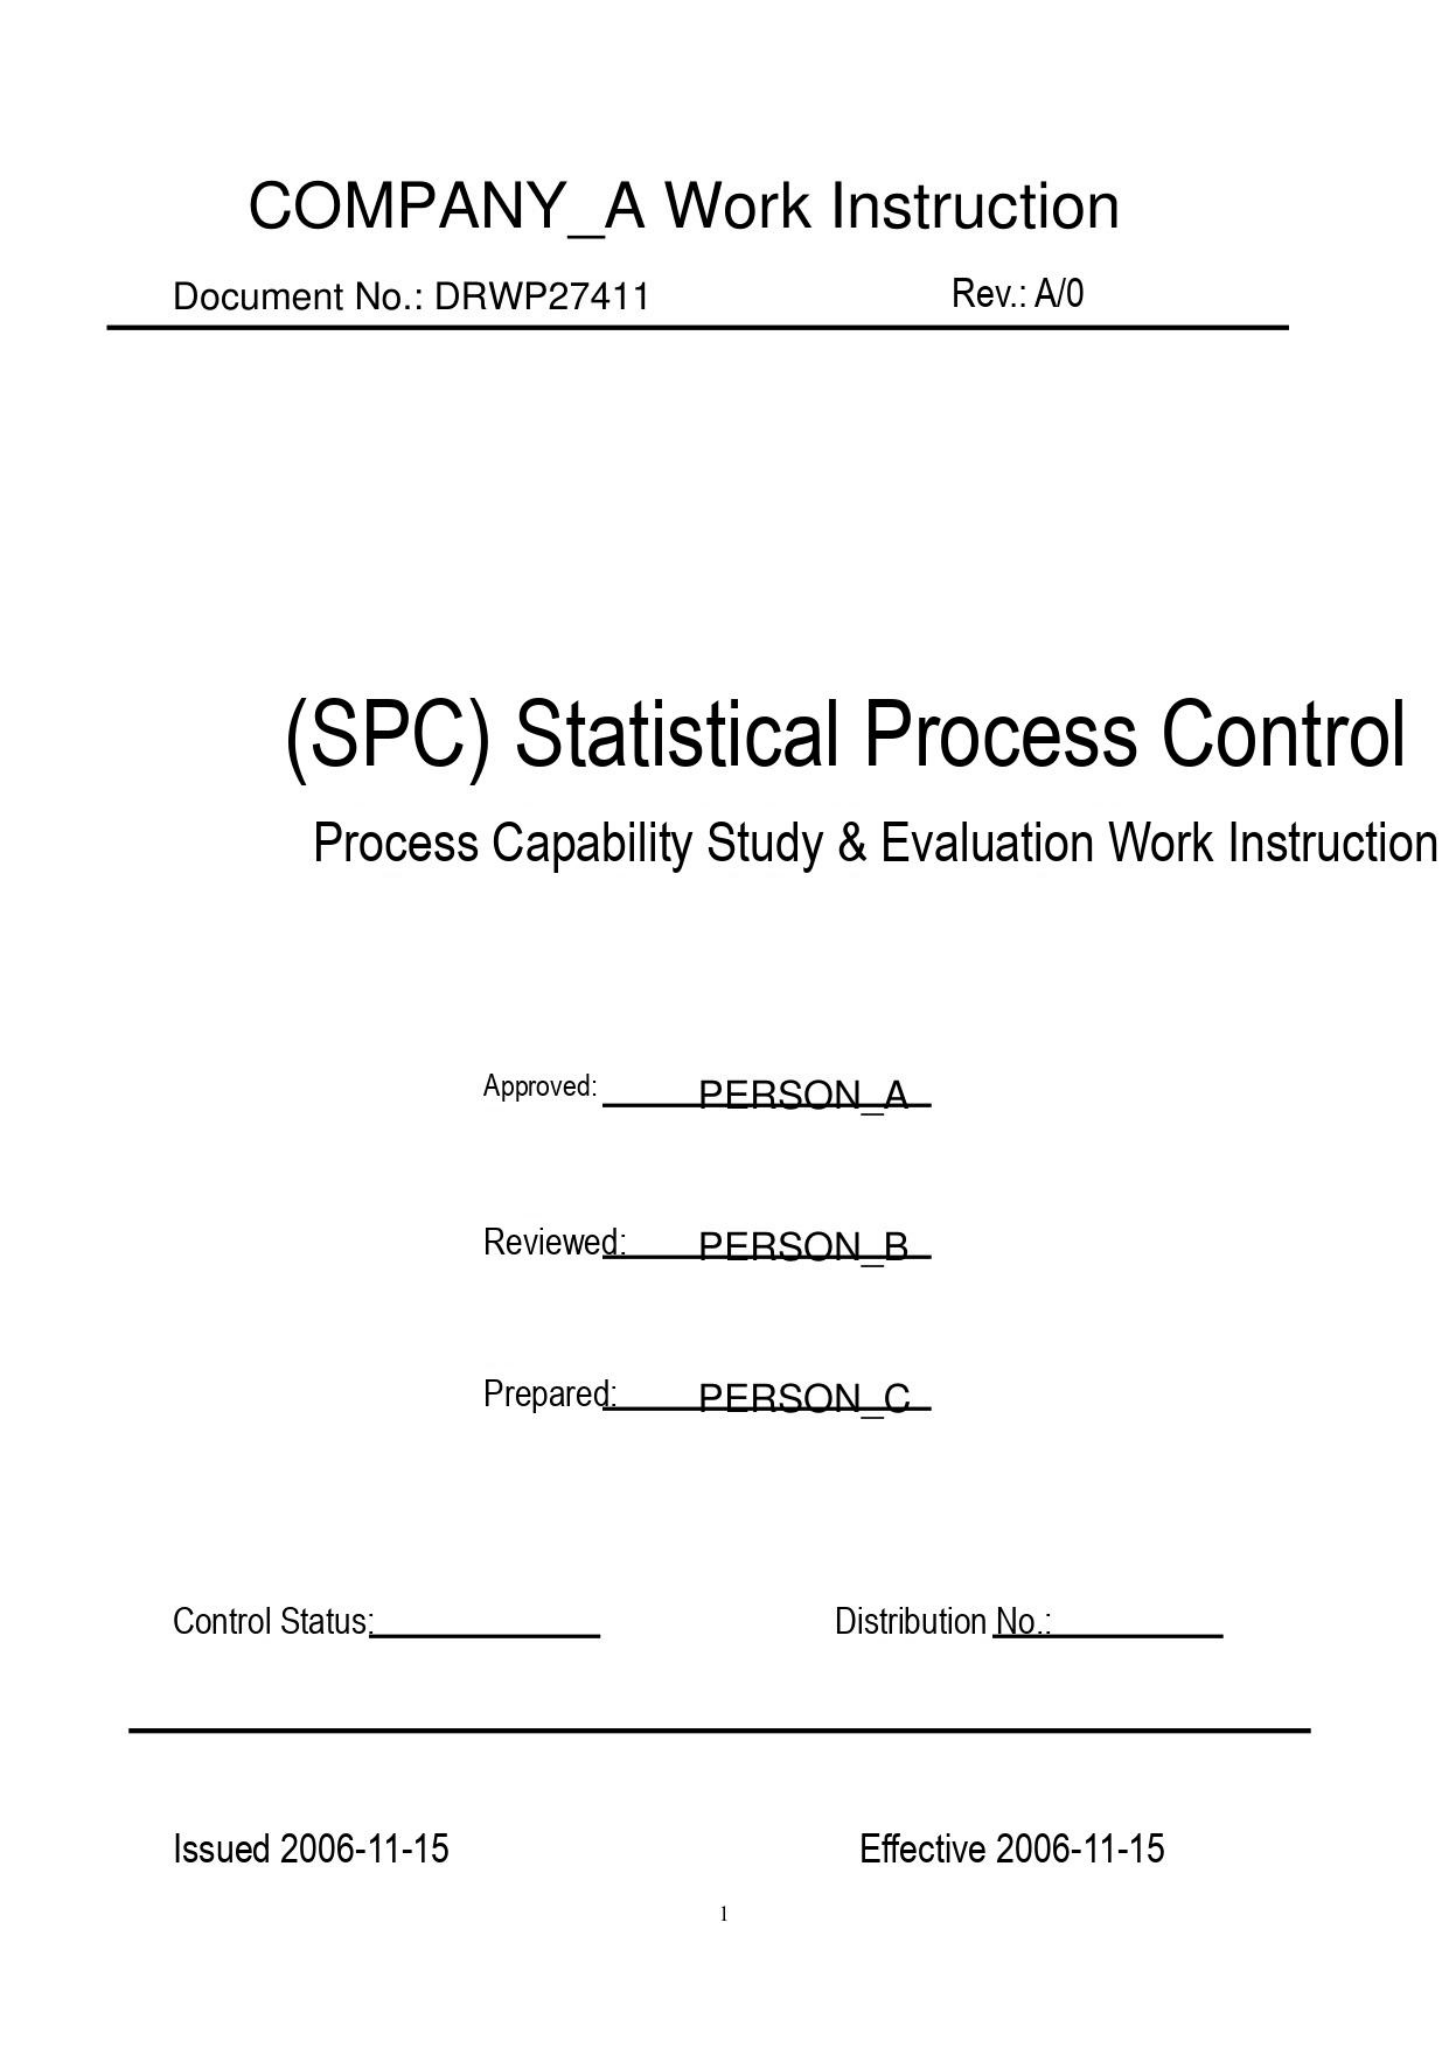COMPANY_A Work Instruction

Document No.: DRWP27411 Rev.: A/0

(SPC) Statistical Process Control

Process Capability Study & Evaluation Work Instruction

Approved: PERSON_A

Reviewed: PERSON_B

Prepared: PERSON_C

Control Status:

Distribution No.:

Issued 2006-11-15

Effective 2006-11-15

1
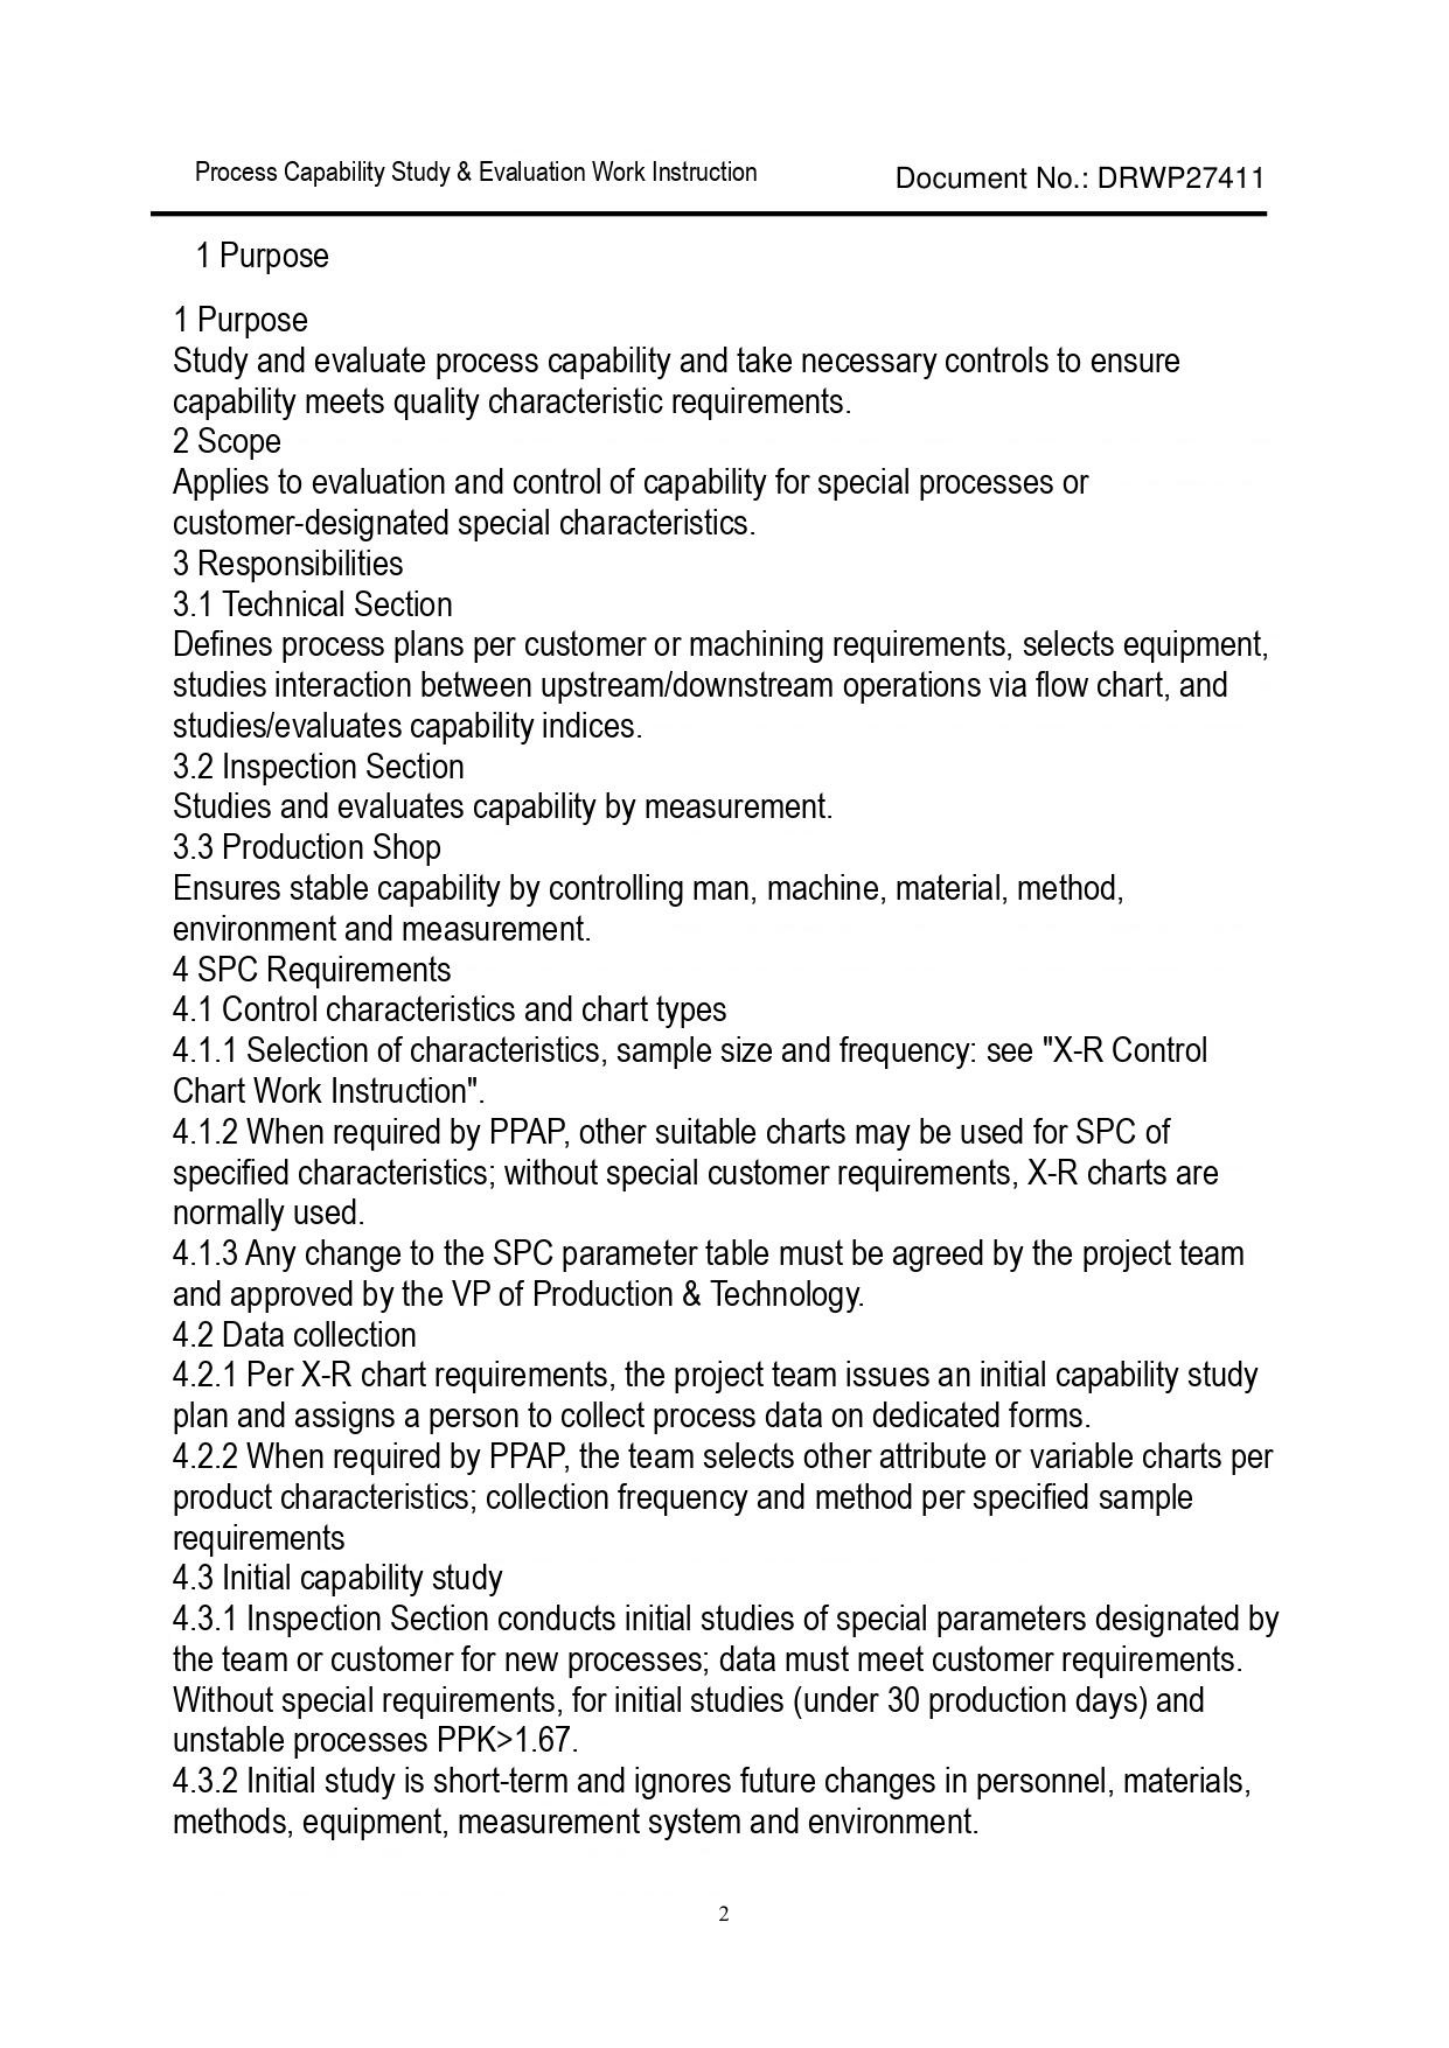Process Capability Study & Evaluation Work Instruction    Document No.: DRWP27411

1 Purpose

1 Purpose
Study and evaluate process capability and take necessary controls to ensure capability meets quality characteristic requirements.
2 Scope
Applies to evaluation and control of capability for special processes or customer-designated special characteristics.
3 Responsibilities
3.1 Technical Section
Defines process plans per customer or machining requirements, selects equipment, studies interaction between upstream/downstream operations via flow chart, and studies/evaluates capability indices.
3.2 Inspection Section
Studies and evaluates capability by measurement.
3.3 Production Shop
Ensures stable capability by controlling man, machine, material, method, environment and measurement.
4 SPC Requirements
4.1 Control characteristics and chart types
4.1.1 Selection of characteristics, sample size and frequency: see "X-R Control Chart Work Instruction".
4.1.2 When required by PPAP, other suitable charts may be used for SPC of specified characteristics; without special customer requirements, X-R charts are normally used.
4.1.3 Any change to the SPC parameter table must be agreed by the project team and approved by the VP of Production & Technology.
4.2 Data collection
4.2.1 Per X-R chart requirements, the project team issues an initial capability study plan and assigns a person to collect process data on dedicated forms.
4.2.2 When required by PPAP, the team selects other attribute or variable charts per product characteristics; collection frequency and method per specified sample requirements
4.3 Initial capability study
4.3.1 Inspection Section conducts initial studies of special parameters designated by the team or customer for new processes; data must meet customer requirements. Without special requirements, for initial studies (under 30 production days) and unstable processes PPK>1.67.
4.3.2 Initial study is short-term and ignores future changes in personnel, materials, methods, equipment, measurement system and environment.

2
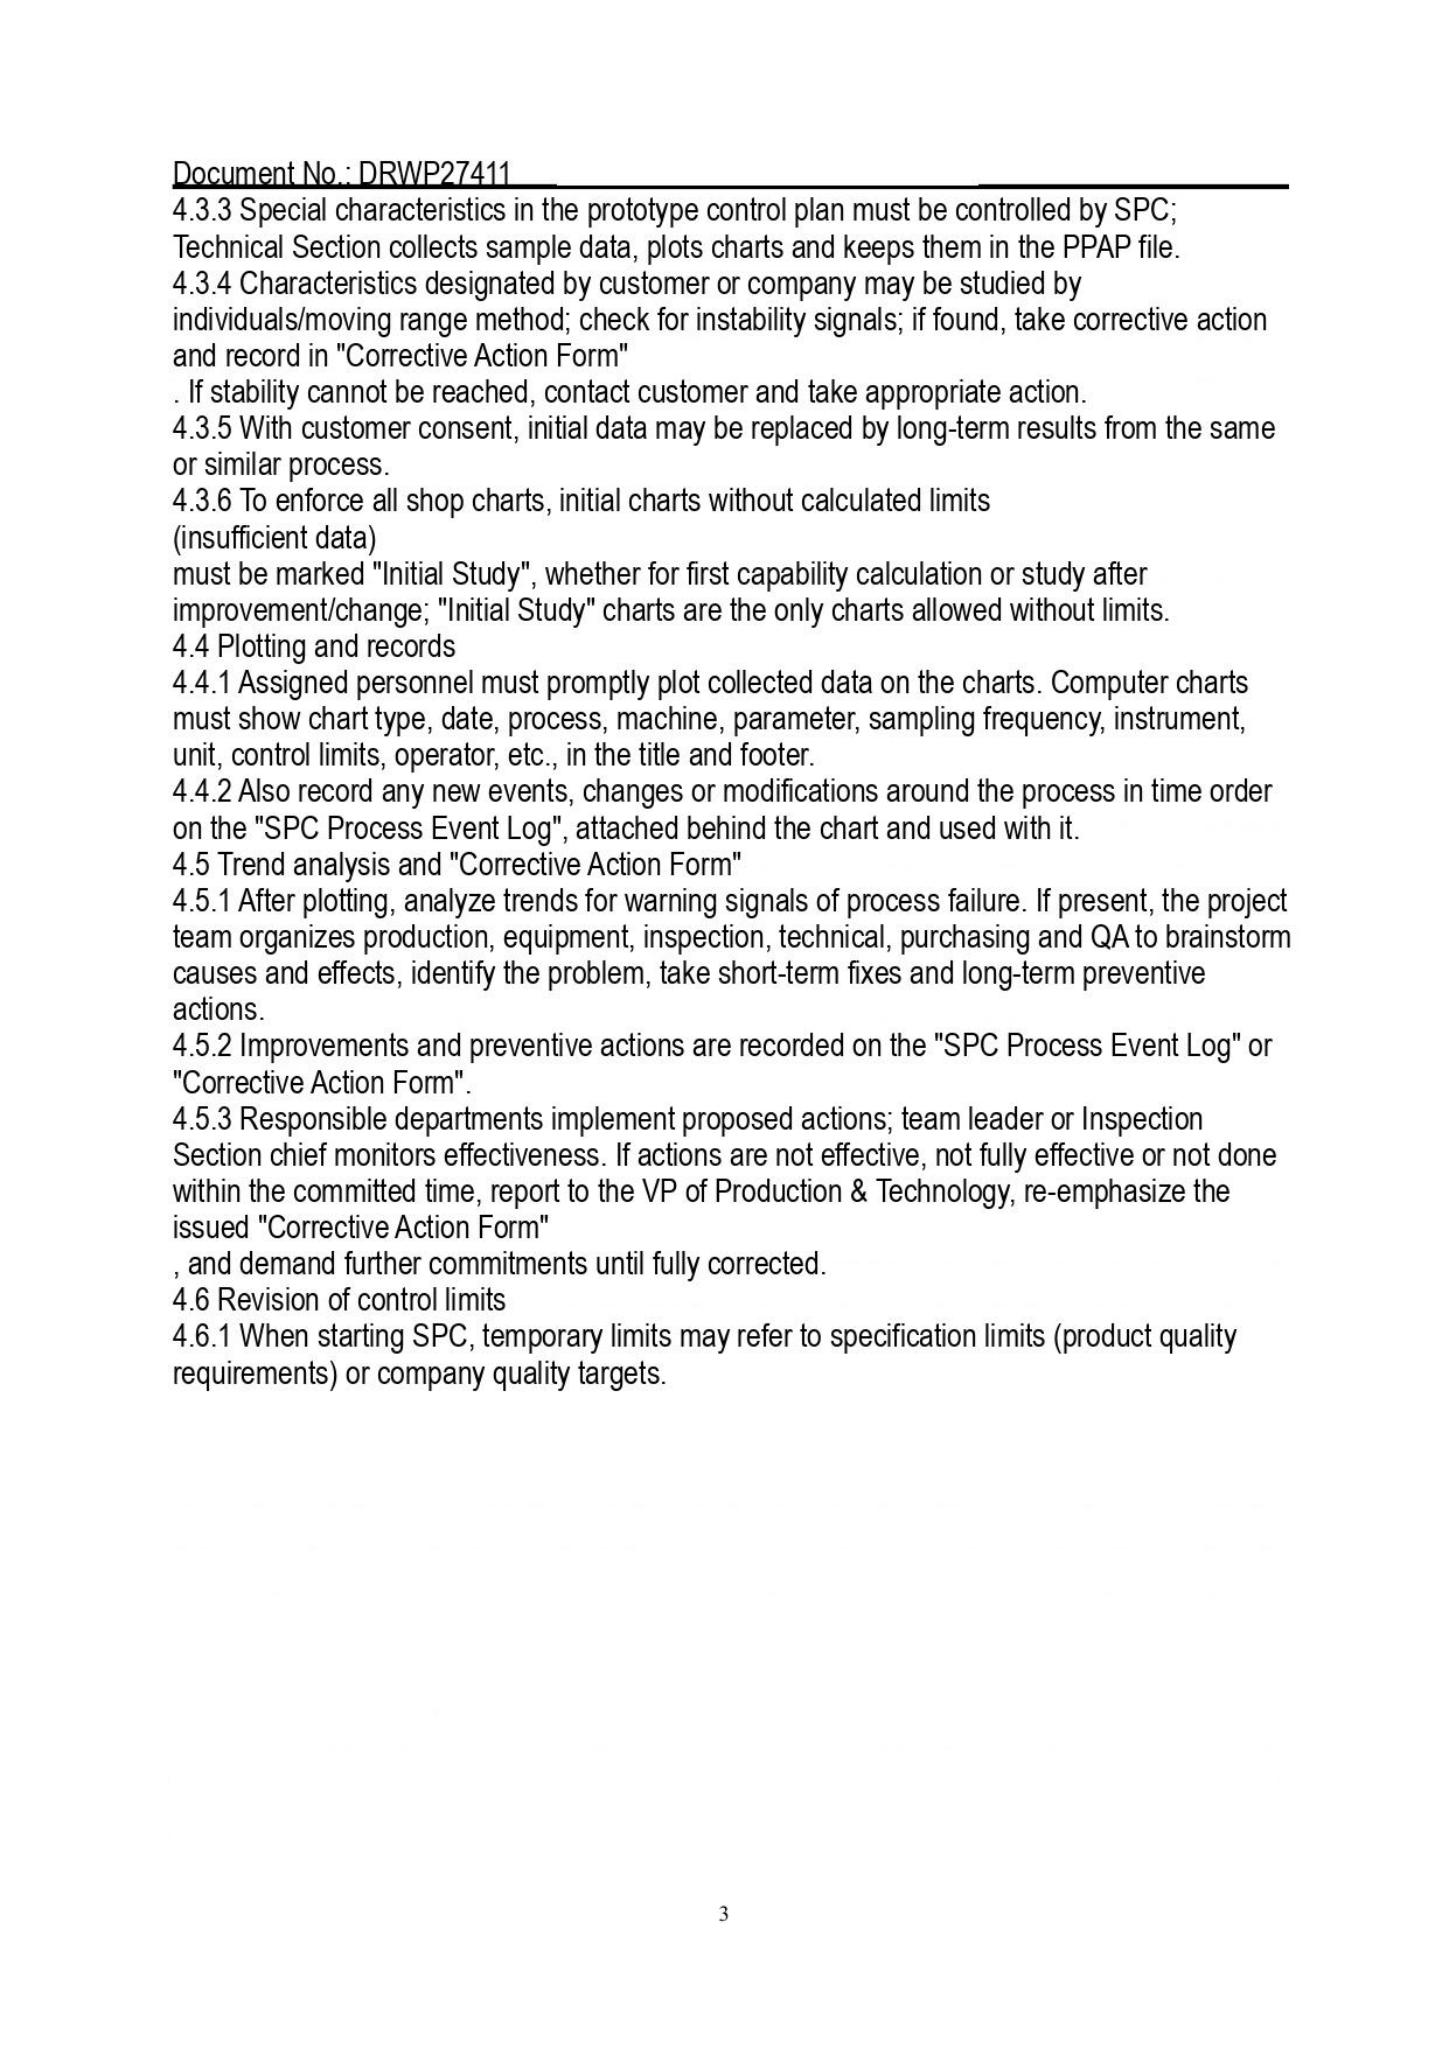Document No.: DRWP27411

4.3.3 Special characteristics in the prototype control plan must be controlled by SPC; Technical Section collects sample data, plots charts and keeps them in the PPAP file.

4.3.4 Characteristics designated by customer or company may be studied by individuals/moving range method; check for instability signals; if found, take corrective action and record in "Corrective Action Form"
. If stability cannot be reached, contact customer and take appropriate action.

4.3.5 With customer consent, initial data may be replaced by long-term results from the same or similar process.

4.3.6 To enforce all shop charts, initial charts without calculated limits
(insufficient data)
must be marked "Initial Study", whether for first capability calculation or study after improvement/change; "Initial Study" charts are the only charts allowed without limits.

4.4 Plotting and records

4.4.1 Assigned personnel must promptly plot collected data on the charts. Computer charts must show chart type, date, process, machine, parameter, sampling frequency, instrument, unit, control limits, operator, etc., in the title and footer.

4.4.2 Also record any new events, changes or modifications around the process in time order on the "SPC Process Event Log", attached behind the chart and used with it.

4.5 Trend analysis and "Corrective Action Form"

4.5.1 After plotting, analyze trends for warning signals of process failure. If present, the project team organizes production, equipment, inspection, technical, purchasing and QA to brainstorm causes and effects, identify the problem, take short-term fixes and long-term preventive actions.

4.5.2 Improvements and preventive actions are recorded on the "SPC Process Event Log" or "Corrective Action Form".

4.5.3 Responsible departments implement proposed actions; team leader or Inspection Section chief monitors effectiveness. If actions are not effective, not fully effective or not done within the committed time, report to the VP of Production & Technology, re-emphasize the issued "Corrective Action Form"
, and demand further commitments until fully corrected.

4.6 Revision of control limits

4.6.1 When starting SPC, temporary limits may refer to specification limits (product quality requirements) or company quality targets.

3
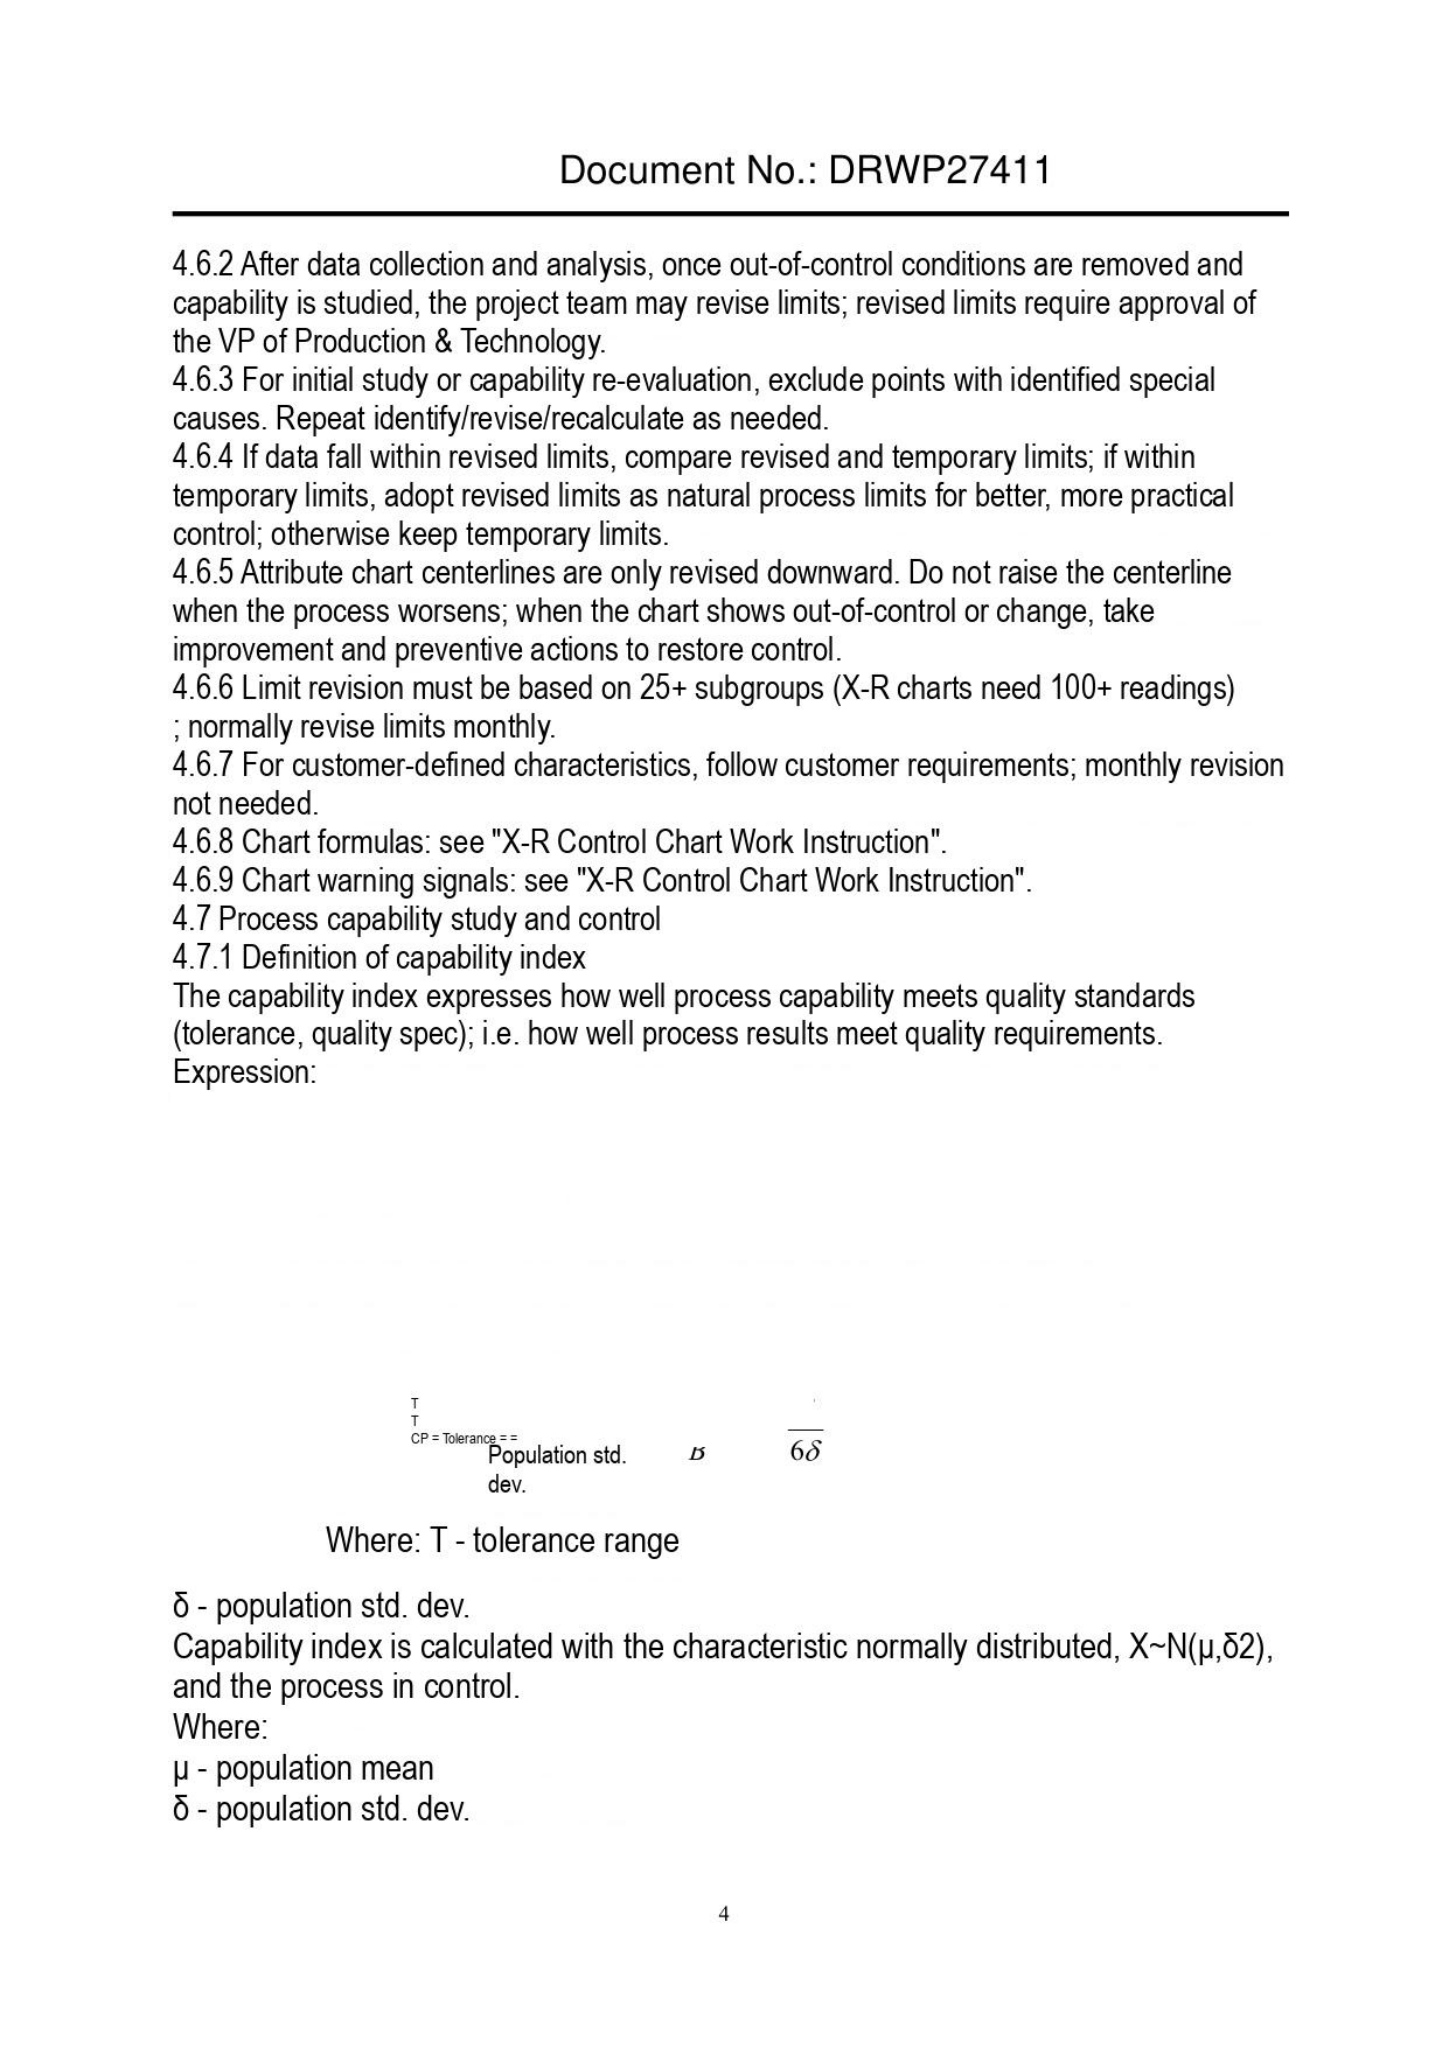Document No.: DRWP27411

4.6.2 After data collection and analysis, once out-of-control conditions are removed and capability is studied, the project team may revise limits; revised limits require approval of the VP of Production & Technology.
4.6.3 For initial study or capability re-evaluation, exclude points with identified special causes. Repeat identify/revise/recalculate as needed.
4.6.4 If data fall within revised limits, compare revised and temporary limits; if within temporary limits, adopt revised limits as natural process limits for better, more practical control; otherwise keep temporary limits.
4.6.5 Attribute chart centerlines are only revised downward. Do not raise the centerline when the process worsens; when the chart shows out-of-control or change, take improvement and preventive actions to restore control.
4.6.6 Limit revision must be based on 25+ subgroups (X-R charts need 100+ readings) ; normally revise limits monthly.
4.6.7 For customer-defined characteristics, follow customer requirements; monthly revision not needed.
4.6.8 Chart formulas: see "X-R Control Chart Work Instruction".
4.6.9 Chart warning signals: see "X-R Control Chart Work Instruction".
4.7 Process capability study and control
4.7.1 Definition of capability index
The capability index expresses how well process capability meets quality standards (tolerance, quality spec); i.e. how well process results meet quality requirements.
Expression:

T
T
CP = Tolerance = =
Population std. dev.　　δ　　6δ

Where: T - tolerance range

δ - population std. dev.
Capability index is calculated with the characteristic normally distributed, X~N(μ,δ2), and the process in control.
Where:
μ - population mean
δ - population std. dev.

4
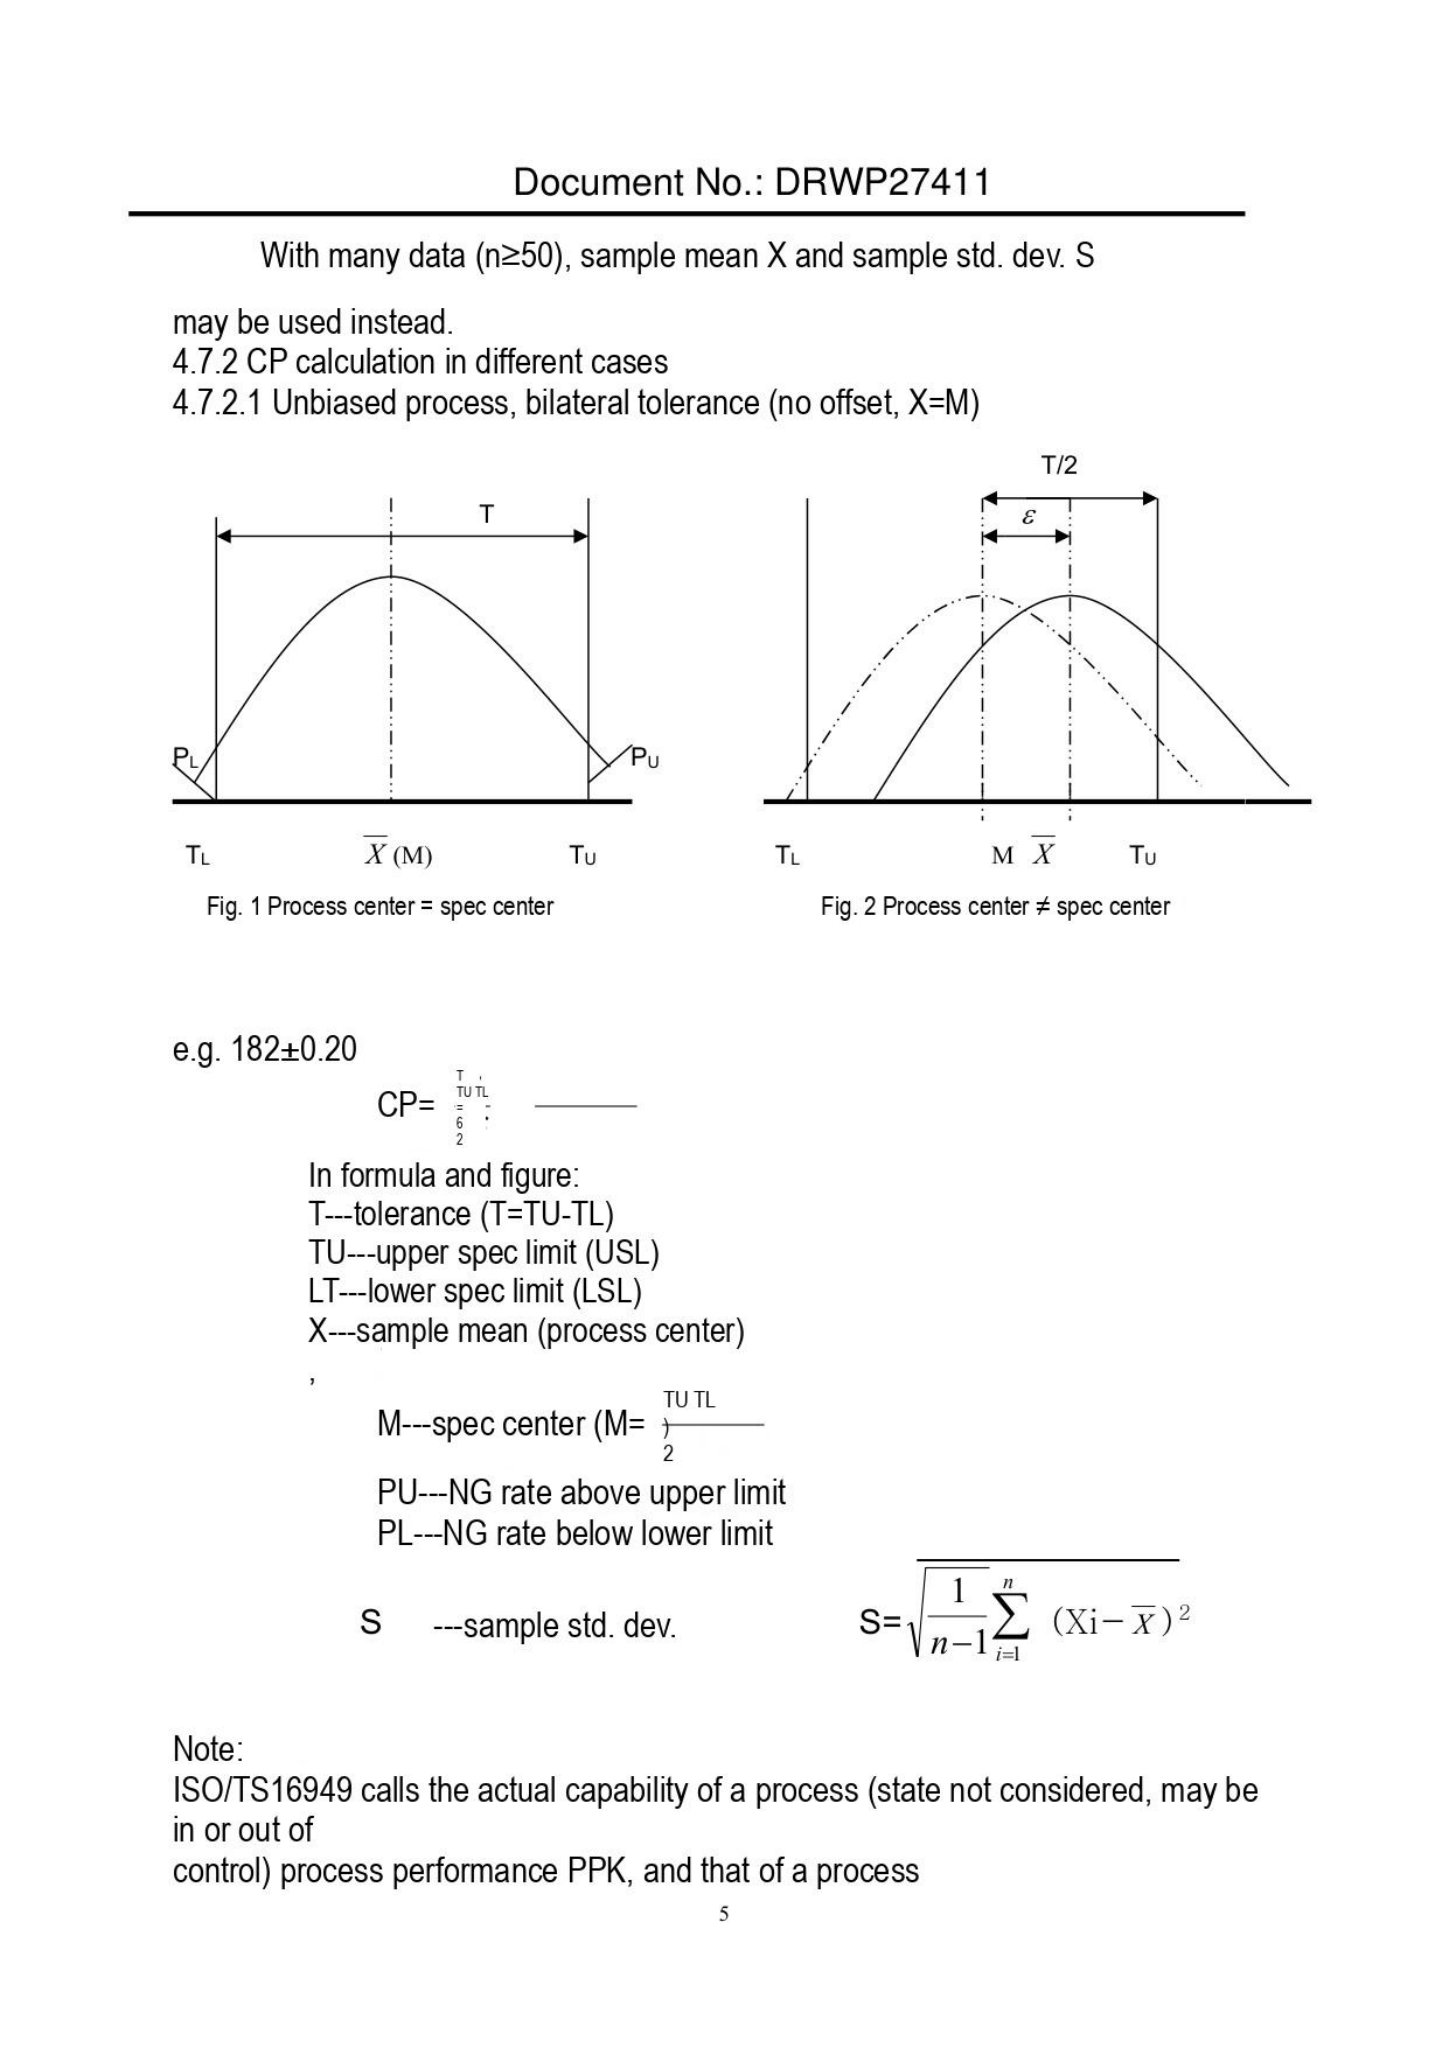Document No.: DRWP27411

With many data (n≥50), sample mean X and sample std. dev. S

may be used instead.
4.7.2 CP calculation in different cases
4.7.2.1 Unbiased process, bilateral tolerance (no offset, X=M)

T

P<sub>L</sub> P<sub>U</sub>

T<sub>L</sub> X̄ (M) T<sub>U</sub>

Fig. 1 Process center = spec center

T/2

ε

T<sub>L</sub> M X̄ T<sub>U</sub>

Fig. 2 Process center ≠ spec center

e.g. 182±0.20

CP= T TU TL = 6 2

In formula and figure:
T---tolerance (T=TU-TL)
TU---upper spec limit (USL)
LT---lower spec limit (LSL)
X---sample mean (process center)
,
M---spec center (M= TU TL ) 2
PU---NG rate above upper limit
PL---NG rate below lower limit

S ---sample std. dev. S=√( 1/(n−1) ∑<sub>i=1</sub><sup>n</sup> (Xi−X̄)<sup>2</sup> )

Note:
ISO/TS16949 calls the actual capability of a process (state not considered, may be in or out of
control) process performance PPK, and that of a process

5
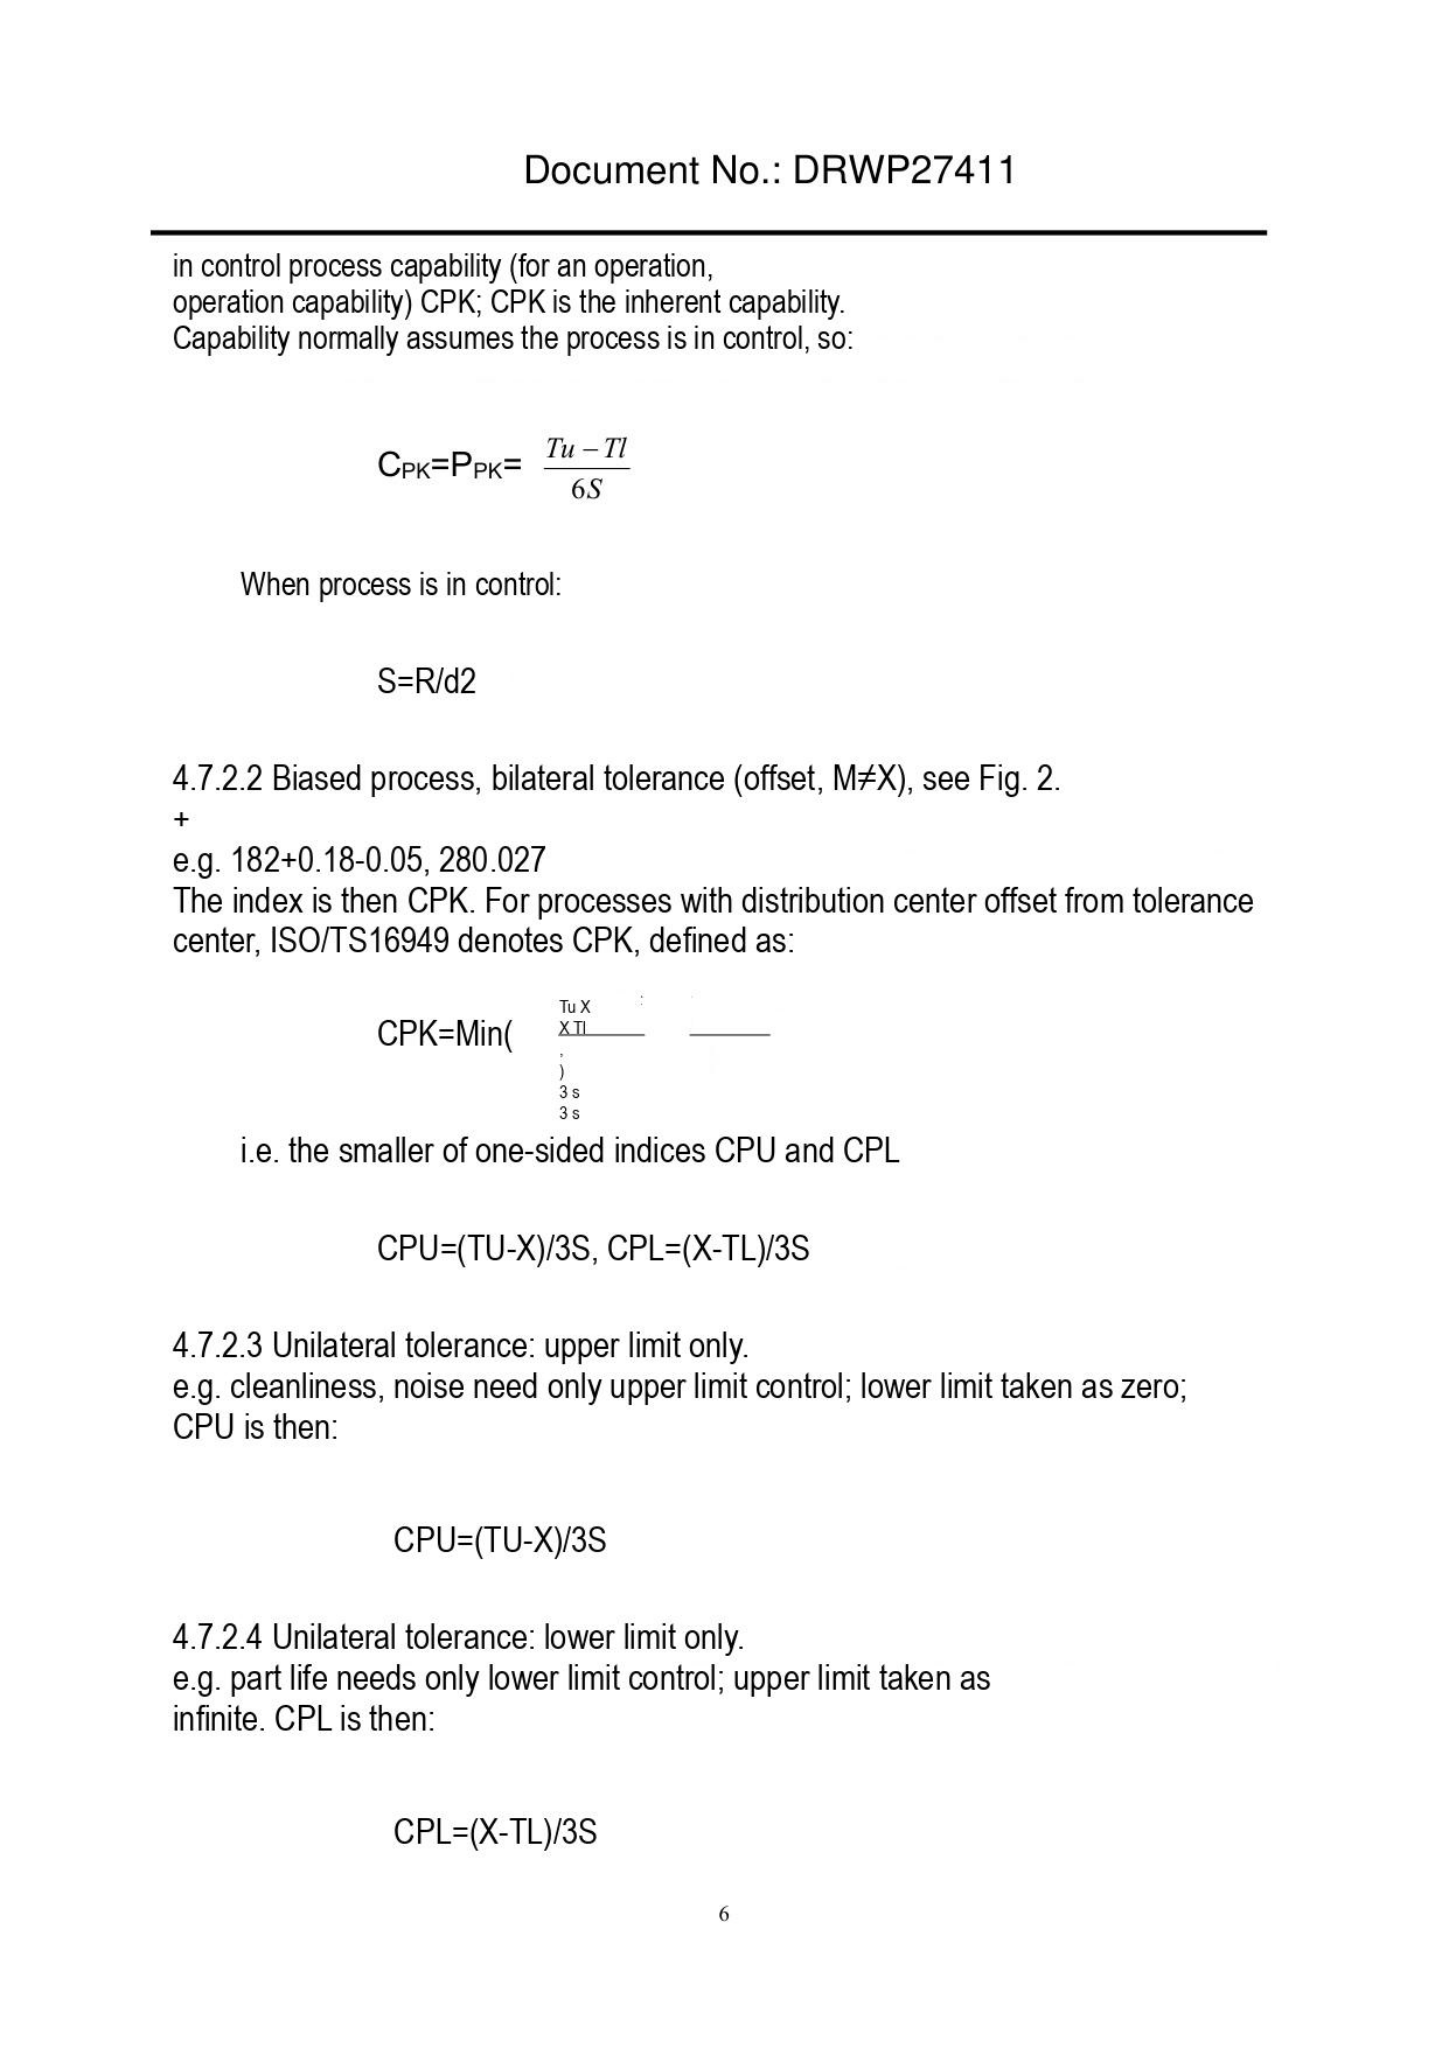Document No.: DRWP27411

in control process capability (for an operation,
operation capability) CPK; CPK is the inherent capability.
Capability normally assumes the process is in control, so:

CPK=PPK= (Tu − Tl)/6S

When process is in control:

S=R/d2

4.7.2.2 Biased process, bilateral tolerance (offset, M≠X), see Fig. 2.
+
e.g. 182+0.18-0.05, 280.027
The index is then CPK. For processes with distribution center offset from tolerance center, ISO/TS16949 denotes CPK, defined as:

CPK=Min(

Tu X
X Tl
,
)
3 s
3 s

i.e. the smaller of one-sided indices CPU and CPL

CPU=(TU-X)/3S, CPL=(X-TL)/3S

4.7.2.3 Unilateral tolerance: upper limit only.
e.g. cleanliness, noise need only upper limit control; lower limit taken as zero;
CPU is then:

CPU=(TU-X)/3S

4.7.2.4 Unilateral tolerance: lower limit only.
e.g. part life needs only lower limit control; upper limit taken as
infinite. CPL is then:

CPL=(X-TL)/3S

6
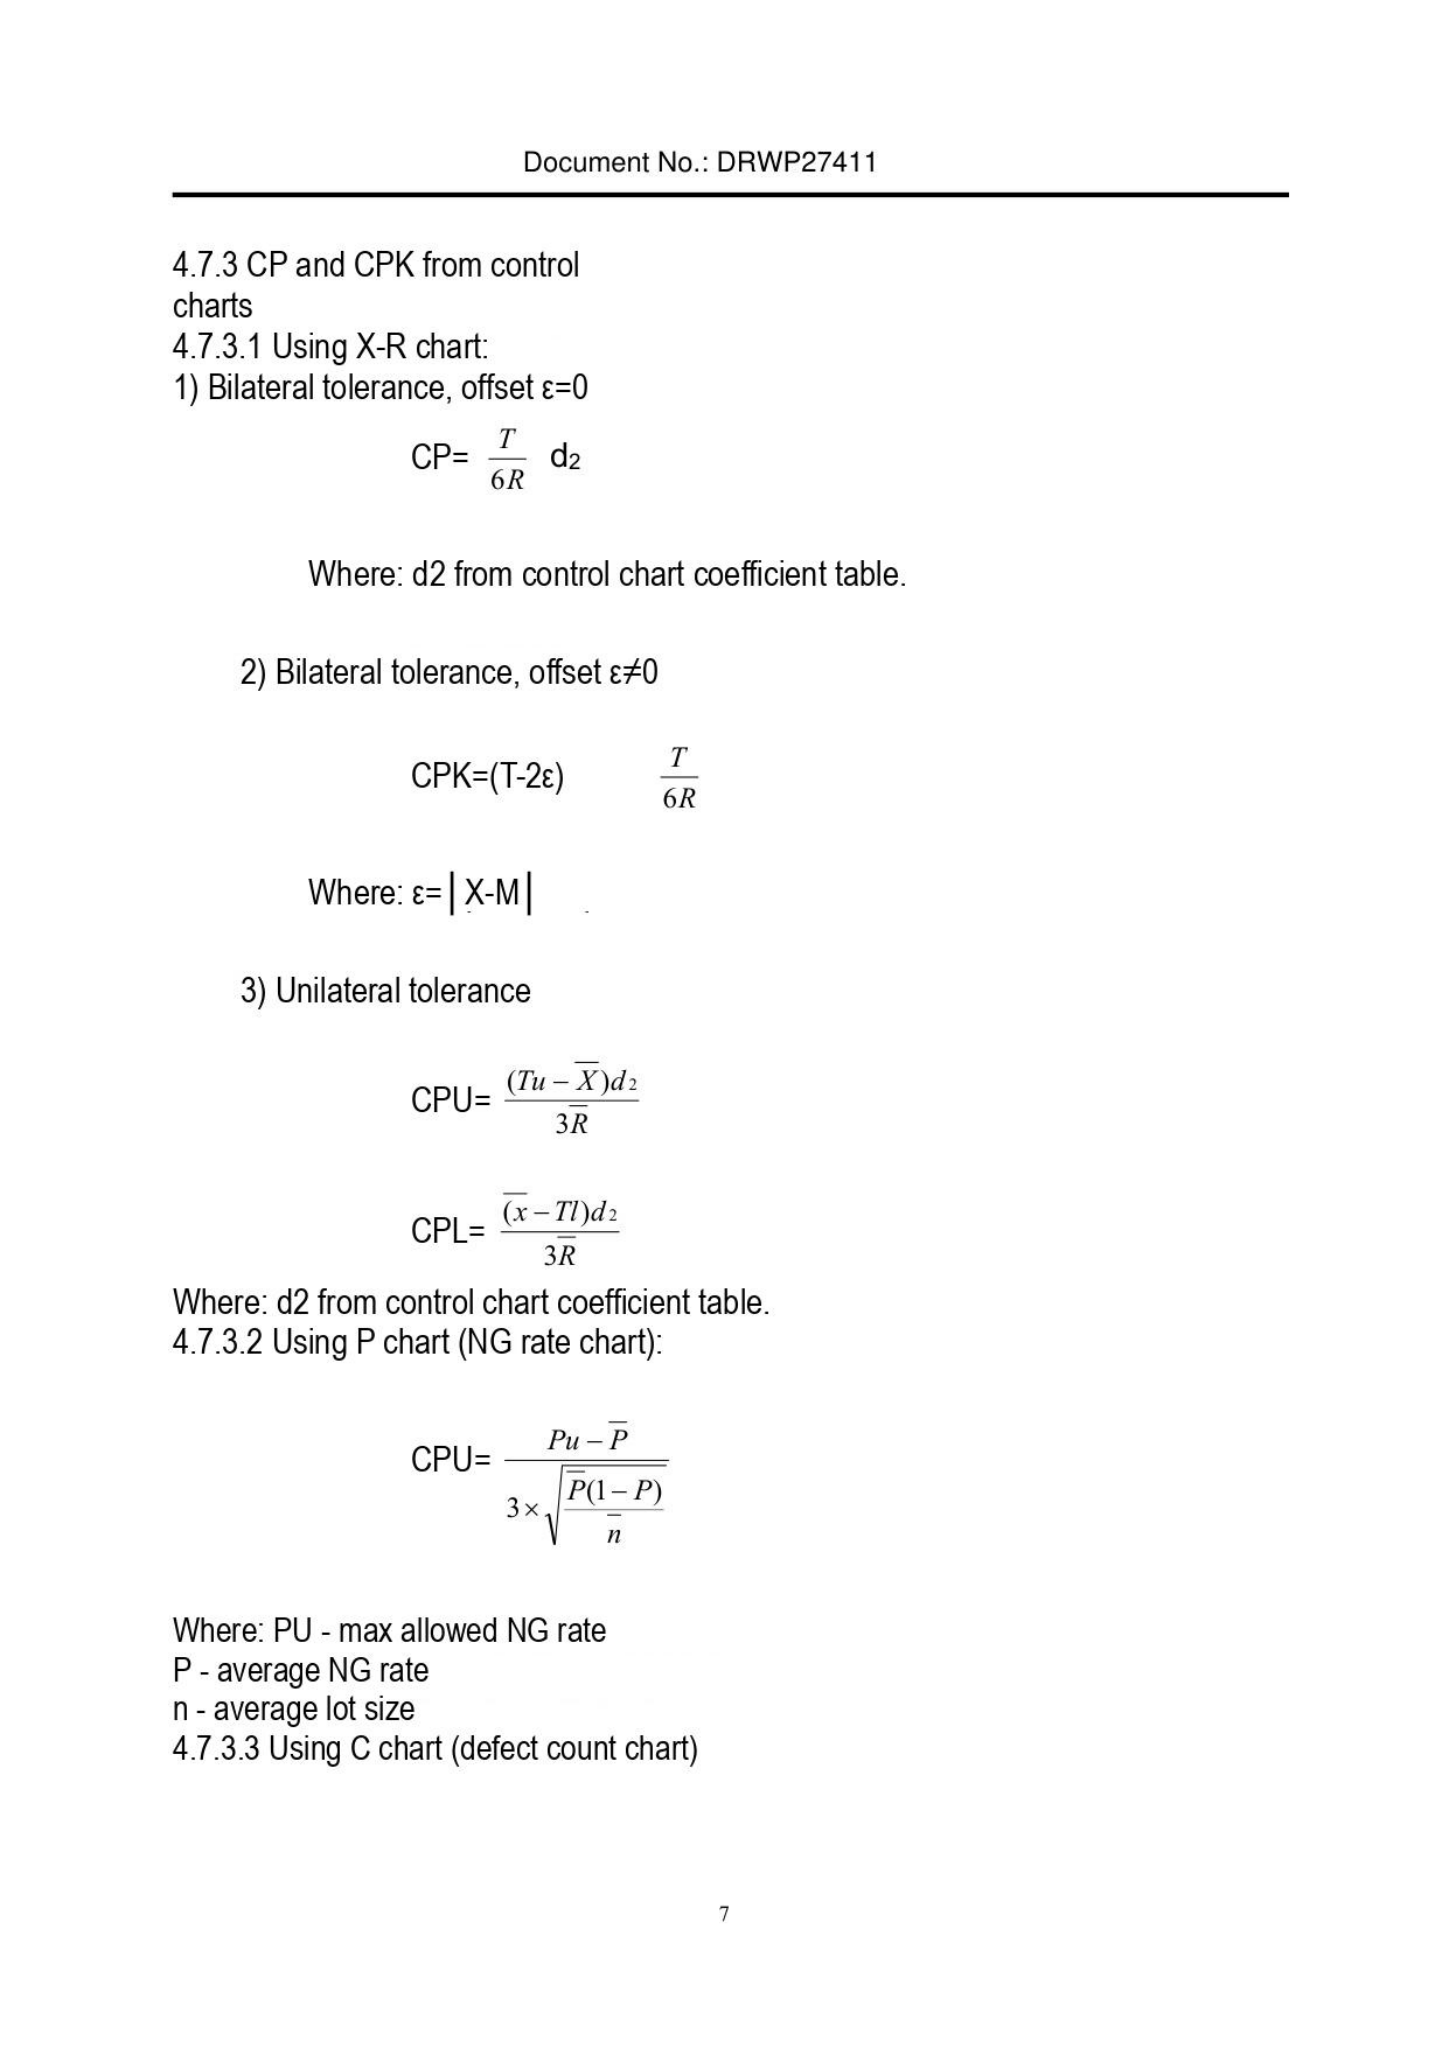Document No.: DRWP27411

4.7.3 CP and CPK from control charts
4.7.3.1 Using X-R chart:
1) Bilateral tolerance, offset ε=0

CP= $\frac{T}{6R}$ d₂

Where: d2 from control chart coefficient table.

2) Bilateral tolerance, offset ε≠0

CPK=(T-2ε) $\frac{T}{6R}$

Where: ε=│X-M│

3) Unilateral tolerance

CPU= $\frac{(Tu-\overline{X})d_2}{3\overline{R}}$

CPL= $\frac{(\overline{x}-Tl)d_2}{3\overline{R}}$

Where: d2 from control chart coefficient table.
4.7.3.2 Using P chart (NG rate chart):

CPU= $\frac{Pu-\overline{P}}{3\times\sqrt{\frac{\overline{P}(1-P)}{\overline{n}}}}$

Where: PU - max allowed NG rate
P - average NG rate
n - average lot size
4.7.3.3 Using C chart (defect count chart)

7